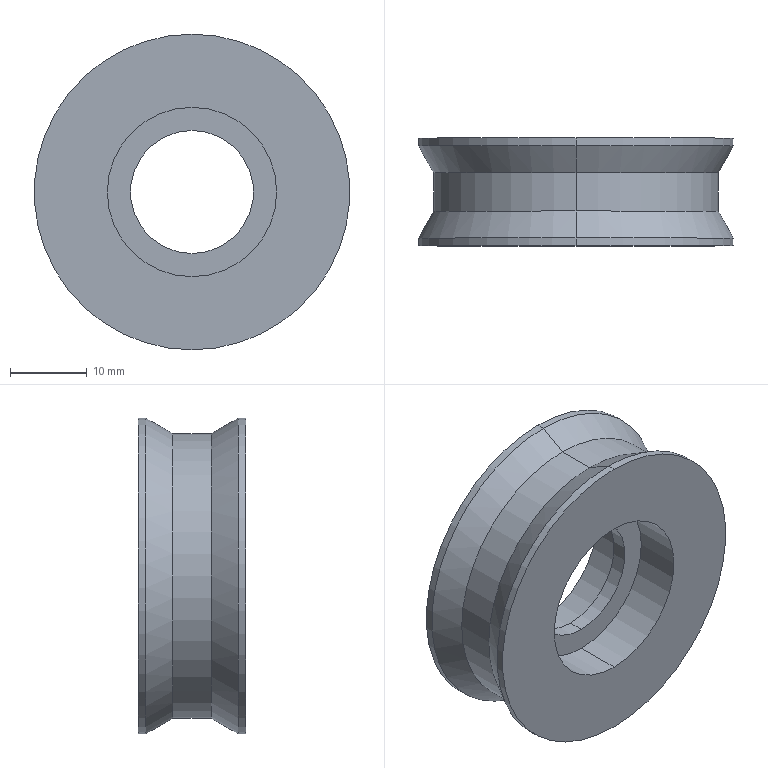Part | SolidWorks | features Revolution 1 | 1 solid | 20 faces | box 41 x 14 x 41 mm | volume 11422 mm3 | cylinder 12 | cone 4 | plane 4 | commonest cylinder face diameters 22 x4 41 x4 16 x2 37 x2
STEP:
#1=CARTESIAN_POINT('',(0.,1.,-11.));
#2=VERTEX_POINT('',#1);
#3=CARTESIAN_POINT('',(0.,1.,11.));
#4=VERTEX_POINT('',#3);
#5=CARTESIAN_POINT('',(0.,1.,0.));
#6=DIRECTION('',(0.,1.,0.));
#7=DIRECTION('',(0.,0.,1.));
#8=AXIS2_PLACEMENT_3D('',#5,#6,#7);
#9=CIRCLE('',#8,11.);
#10=EDGE_CURVE('',#2,#4,#9,.T.);
#11=ORIENTED_EDGE('',*,*,#10,.F.);
#12=CARTESIAN_POINT('',(0.,7.,-11.));
#13=VERTEX_POINT('',#12);
#14=CARTESIAN_POINT('',(0.,20.639,-11.));
#15=DIRECTION('',(0.,1.,0.));
#16=VECTOR('',#15,1000.);
#17=LINE('',#14,#16);
#18=EDGE_CURVE('',#2,#13,#17,.T.);
#19=ORIENTED_EDGE('',*,*,#18,.T.);
#20=CARTESIAN_POINT('',(0.,7.,11.));
#21=VERTEX_POINT('',#20);
#22=CARTESIAN_POINT('',(0.,7.,0.));
#23=DIRECTION('',(0.,1.,0.));
#24=DIRECTION('',(0.,0.,1.));
#25=AXIS2_PLACEMENT_3D('',#22,#23,#24);
#26=CIRCLE('',#25,11.);
#27=EDGE_CURVE('',#13,#21,#26,.T.);
#28=ORIENTED_EDGE('',*,*,#27,.T.);
#29=CARTESIAN_POINT('',(0.,20.639,11.));
#30=DIRECTION('',(0.,1.,0.));
#31=VECTOR('',#30,1000.);
#32=LINE('',#29,#31);
#33=EDGE_CURVE('',#4,#21,#32,.T.);
#34=ORIENTED_EDGE('',*,*,#33,.F.);
#35=EDGE_LOOP('',(#11,#19,#28,#34));
#36=FACE_OUTER_BOUND('',#35,.T.);
#37=CARTESIAN_POINT('',(0.,20.639,0.));
#38=DIRECTION('',(0.,1.,0.));
#39=DIRECTION('',(0.,0.,1.));
#40=AXIS2_PLACEMENT_3D('',#37,#38,#39);
#41=CYLINDRICAL_SURFACE('',#40,11.);
#42=ADVANCED_FACE('',(#36),#41,.F.);
#43=CARTESIAN_POINT('',(0.,-1.,-8.));
#44=VERTEX_POINT('',#43);
#45=CARTESIAN_POINT('',(0.,-1.,8.));
#46=VERTEX_POINT('',#45);
#47=CARTESIAN_POINT('',(0.,-1.,0.));
#48=DIRECTION('',(0.,1.,0.));
#49=DIRECTION('',(0.,0.,1.));
#50=AXIS2_PLACEMENT_3D('',#47,#48,#49);
#51=CIRCLE('',#50,8.);
#52=EDGE_CURVE('',#44,#46,#51,.T.);
#53=ORIENTED_EDGE('',*,*,#52,.F.);
#54=CARTESIAN_POINT('',(0.,1.,-8.));
#55=VERTEX_POINT('',#54);
#56=CARTESIAN_POINT('',(0.,20.639,-8.));
#57=DIRECTION('',(0.,1.,0.));
#58=VECTOR('',#57,1000.);
#59=LINE('',#56,#58);
#60=EDGE_CURVE('',#44,#55,#59,.T.);
#61=ORIENTED_EDGE('',*,*,#60,.T.);
#62=CARTESIAN_POINT('',(0.,1.,8.));
#63=VERTEX_POINT('',#62);
#64=CARTESIAN_POINT('',(0.,1.,0.));
#65=DIRECTION('',(0.,1.,0.));
#66=DIRECTION('',(0.,0.,1.));
#67=AXIS2_PLACEMENT_3D('',#64,#65,#66);
#68=CIRCLE('',#67,8.);
#69=EDGE_CURVE('',#55,#63,#68,.T.);
#70=ORIENTED_EDGE('',*,*,#69,.T.);
#71=CARTESIAN_POINT('',(0.,20.639,8.));
#72=DIRECTION('',(0.,1.,0.));
#73=VECTOR('',#72,1000.);
#74=LINE('',#71,#73);
#75=EDGE_CURVE('',#46,#63,#74,.T.);
#76=ORIENTED_EDGE('',*,*,#75,.F.);
#77=EDGE_LOOP('',(#53,#61,#70,#76));
#78=FACE_OUTER_BOUND('',#77,.T.);
#79=CARTESIAN_POINT('',(0.,20.639,0.));
#80=DIRECTION('',(0.,1.,0.));
#81=DIRECTION('',(0.,0.,1.));
#82=AXIS2_PLACEMENT_3D('',#79,#80,#81);
#83=CYLINDRICAL_SURFACE('',#82,8.);
#84=ADVANCED_FACE('',(#78),#83,.F.);
#85=CARTESIAN_POINT('',(0.,-7.,-11.));
#86=VERTEX_POINT('',#85);
#87=CARTESIAN_POINT('',(0.,-7.,11.));
#88=VERTEX_POINT('',#87);
#89=CARTESIAN_POINT('',(0.,-7.,0.));
#90=DIRECTION('',(0.,1.,0.));
#91=DIRECTION('',(0.,0.,1.));
#92=AXIS2_PLACEMENT_3D('',#89,#90,#91);
#93=CIRCLE('',#92,11.);
#94=EDGE_CURVE('',#86,#88,#93,.T.);
#95=ORIENTED_EDGE('',*,*,#94,.F.);
#96=CARTESIAN_POINT('',(0.,-1.,-11.));
#97=VERTEX_POINT('',#96);
#98=CARTESIAN_POINT('',(0.,20.639,-11.));
#99=DIRECTION('',(0.,1.,0.));
#100=VECTOR('',#99,1000.);
#101=LINE('',#98,#100);
#102=EDGE_CURVE('',#86,#97,#101,.T.);
#103=ORIENTED_EDGE('',*,*,#102,.T.);
#104=CARTESIAN_POINT('',(0.,-1.,11.));
#105=VERTEX_POINT('',#104);
#106=CARTESIAN_POINT('',(0.,-1.,0.));
#107=DIRECTION('',(0.,1.,0.));
#108=DIRECTION('',(0.,0.,1.));
#109=AXIS2_PLACEMENT_3D('',#106,#107,#108);
#110=CIRCLE('',#109,11.);
#111=EDGE_CURVE('',#97,#105,#110,.T.);
#112=ORIENTED_EDGE('',*,*,#111,.T.);
#113=CARTESIAN_POINT('',(0.,20.639,11.));
#114=DIRECTION('',(0.,1.,0.));
#115=VECTOR('',#114,1000.);
#116=LINE('',#113,#115);
#117=EDGE_CURVE('',#88,#105,#116,.T.);
#118=ORIENTED_EDGE('',*,*,#117,.F.);
#119=EDGE_LOOP('',(#95,#103,#112,#118));
#120=FACE_OUTER_BOUND('',#119,.T.);
#121=CARTESIAN_POINT('',(0.,20.639,0.));
#122=DIRECTION('',(0.,1.,0.));
#123=DIRECTION('',(0.,0.,1.));
#124=AXIS2_PLACEMENT_3D('',#121,#122,#123);
#125=CYLINDRICAL_SURFACE('',#124,11.);
#126=ADVANCED_FACE('',(#120),#125,.F.);
#127=CARTESIAN_POINT('',(0.,-7.,20.5));
#128=VERTEX_POINT('',#127);
#129=CARTESIAN_POINT('',(0.,-7.,-20.5));
#130=VERTEX_POINT('',#129);
#131=CARTESIAN_POINT('',(0.,-7.,0.));
#132=DIRECTION('',(0.,1.,0.));
#133=DIRECTION('',(0.,0.,1.));
#134=AXIS2_PLACEMENT_3D('',#131,#132,#133);
#135=CIRCLE('',#134,20.5);
#136=EDGE_CURVE('',#128,#130,#135,.T.);
#137=ORIENTED_EDGE('',*,*,#136,.T.);
#138=CARTESIAN_POINT('',(0.,-6.,-20.5));
#139=VERTEX_POINT('',#138);
#140=CARTESIAN_POINT('',(0.,20.639,-20.5));
#141=DIRECTION('',(0.,1.,0.));
#142=VECTOR('',#141,1000.);
#143=LINE('',#140,#142);
#144=EDGE_CURVE('',#130,#139,#143,.T.);
#145=ORIENTED_EDGE('',*,*,#144,.T.);
#146=CARTESIAN_POINT('',(0.,-6.,20.5));
#147=VERTEX_POINT('',#146);
#148=CARTESIAN_POINT('',(0.,-6.,0.));
#149=DIRECTION('',(0.,1.,0.));
#150=DIRECTION('',(0.,0.,1.));
#151=AXIS2_PLACEMENT_3D('',#148,#149,#150);
#152=CIRCLE('',#151,20.5);
#153=EDGE_CURVE('',#147,#139,#152,.T.);
#154=ORIENTED_EDGE('',*,*,#153,.F.);
#155=CARTESIAN_POINT('',(0.,20.639,20.5));
#156=DIRECTION('',(0.,1.,0.));
#157=VECTOR('',#156,1000.);
#158=LINE('',#155,#157);
#159=EDGE_CURVE('',#128,#147,#158,.T.);
#160=ORIENTED_EDGE('',*,*,#159,.F.);
#161=EDGE_LOOP('',(#137,#145,#154,#160));
#162=FACE_OUTER_BOUND('',#161,.T.);
#163=CARTESIAN_POINT('',(0.,20.639,0.));
#164=DIRECTION('',(0.,1.,0.));
#165=DIRECTION('',(0.,0.,1.));
#166=AXIS2_PLACEMENT_3D('',#163,#164,#165);
#167=CYLINDRICAL_SURFACE('',#166,20.5);
#168=ADVANCED_FACE('',(#162),#167,.T.);
#169=CARTESIAN_POINT('',(0.,-2.5,18.5));
#170=VERTEX_POINT('',#169);
#171=CARTESIAN_POINT('',(0.,-2.5,-18.5));
#172=VERTEX_POINT('',#171);
#173=CARTESIAN_POINT('',(0.,-2.5,0.));
#174=DIRECTION('',(0.,1.,0.));
#175=DIRECTION('',(0.,0.,1.));
#176=AXIS2_PLACEMENT_3D('',#173,#174,#175);
#177=CIRCLE('',#176,18.5);
#178=EDGE_CURVE('',#170,#172,#177,.T.);
#179=ORIENTED_EDGE('',*,*,#178,.F.);
#180=CARTESIAN_POINT('',(0.,-6.,20.5));
#181=DIRECTION('',(0.,-0.8682,0.4961));
#182=VECTOR('',#181,1000.);
#183=LINE('',#180,#182);
#184=EDGE_CURVE('',#170,#147,#183,.T.);
#185=ORIENTED_EDGE('',*,*,#184,.T.);
#186=ORIENTED_EDGE('',*,*,#153,.T.);
#187=CARTESIAN_POINT('',(0.,-6.,-20.5));
#188=DIRECTION('',(0.,-0.8682,-0.4961));
#189=VECTOR('',#188,1000.);
#190=LINE('',#187,#189);
#191=EDGE_CURVE('',#172,#139,#190,.T.);
#192=ORIENTED_EDGE('',*,*,#191,.F.);
#193=EDGE_LOOP('',(#179,#185,#186,#192));
#194=FACE_OUTER_BOUND('',#193,.T.);
#195=CARTESIAN_POINT('',(0.,-6.,0.));
#196=DIRECTION('',(0.,-1.,0.));
#197=DIRECTION('',(0.,0.,-1.));
#198=AXIS2_PLACEMENT_3D('',#195,#196,#197);
#199=CONICAL_SURFACE('',#198,20.5,0.5191);
#200=ADVANCED_FACE('',(#194),#199,.T.);
#201=ORIENTED_EDGE('',*,*,#178,.T.);
#202=CARTESIAN_POINT('',(0.,2.5,-18.5));
#203=VERTEX_POINT('',#202);
#204=CARTESIAN_POINT('',(0.,20.639,-18.5));
#205=DIRECTION('',(0.,1.,0.));
#206=VECTOR('',#205,1000.);
#207=LINE('',#204,#206);
#208=EDGE_CURVE('',#172,#203,#207,.T.);
#209=ORIENTED_EDGE('',*,*,#208,.T.);
#210=CARTESIAN_POINT('',(0.,2.5,18.5));
#211=VERTEX_POINT('',#210);
#212=CARTESIAN_POINT('',(0.,2.5,0.));
#213=DIRECTION('',(0.,1.,0.));
#214=DIRECTION('',(0.,0.,1.));
#215=AXIS2_PLACEMENT_3D('',#212,#213,#214);
#216=CIRCLE('',#215,18.5);
#217=EDGE_CURVE('',#211,#203,#216,.T.);
#218=ORIENTED_EDGE('',*,*,#217,.F.);
#219=CARTESIAN_POINT('',(0.,20.639,18.5));
#220=DIRECTION('',(0.,1.,0.));
#221=VECTOR('',#220,1000.);
#222=LINE('',#219,#221);
#223=EDGE_CURVE('',#170,#211,#222,.T.);
#224=ORIENTED_EDGE('',*,*,#223,.F.);
#225=EDGE_LOOP('',(#201,#209,#218,#224));
#226=FACE_OUTER_BOUND('',#225,.T.);
#227=CARTESIAN_POINT('',(0.,20.639,0.));
#228=DIRECTION('',(0.,1.,0.));
#229=DIRECTION('',(0.,0.,1.));
#230=AXIS2_PLACEMENT_3D('',#227,#228,#229);
#231=CYLINDRICAL_SURFACE('',#230,18.5);
#232=ADVANCED_FACE('',(#226),#231,.T.);
#233=ORIENTED_EDGE('',*,*,#217,.T.);
#234=CARTESIAN_POINT('',(0.,6.,-20.5));
#235=VERTEX_POINT('',#234);
#236=CARTESIAN_POINT('',(0.,2.5,-18.5));
#237=DIRECTION('',(0.,0.8682,-0.4961));
#238=VECTOR('',#237,1000.);
#239=LINE('',#236,#238);
#240=EDGE_CURVE('',#203,#235,#239,.T.);
#241=ORIENTED_EDGE('',*,*,#240,.T.);
#242=CARTESIAN_POINT('',(0.,6.,20.5));
#243=VERTEX_POINT('',#242);
#244=CARTESIAN_POINT('',(0.,6.,0.));
#245=DIRECTION('',(0.,1.,0.));
#246=DIRECTION('',(0.,0.,1.));
#247=AXIS2_PLACEMENT_3D('',#244,#245,#246);
#248=CIRCLE('',#247,20.5);
#249=EDGE_CURVE('',#243,#235,#248,.T.);
#250=ORIENTED_EDGE('',*,*,#249,.F.);
#251=CARTESIAN_POINT('',(0.,2.5,18.5));
#252=DIRECTION('',(0.,0.8682,0.4961));
#253=VECTOR('',#252,1000.);
#254=LINE('',#251,#253);
#255=EDGE_CURVE('',#211,#243,#254,.T.);
#256=ORIENTED_EDGE('',*,*,#255,.F.);
#257=EDGE_LOOP('',(#233,#241,#250,#256));
#258=FACE_OUTER_BOUND('',#257,.T.);
#259=CARTESIAN_POINT('',(0.,2.5,0.));
#260=DIRECTION('',(0.,1.,0.));
#261=DIRECTION('',(0.,0.,1.));
#262=AXIS2_PLACEMENT_3D('',#259,#260,#261);
#263=CONICAL_SURFACE('',#262,18.5,0.5191);
#264=ADVANCED_FACE('',(#258),#263,.T.);
#265=ORIENTED_EDGE('',*,*,#249,.T.);
#266=CARTESIAN_POINT('',(0.,7.,-20.5));
#267=VERTEX_POINT('',#266);
#268=CARTESIAN_POINT('',(0.,20.639,-20.5));
#269=DIRECTION('',(0.,1.,0.));
#270=VECTOR('',#269,1000.);
#271=LINE('',#268,#270);
#272=EDGE_CURVE('',#235,#267,#271,.T.);
#273=ORIENTED_EDGE('',*,*,#272,.T.);
#274=CARTESIAN_POINT('',(0.,7.,20.5));
#275=VERTEX_POINT('',#274);
#276=CARTESIAN_POINT('',(0.,7.,0.));
#277=DIRECTION('',(0.,1.,0.));
#278=DIRECTION('',(0.,0.,1.));
#279=AXIS2_PLACEMENT_3D('',#276,#277,#278);
#280=CIRCLE('',#279,20.5);
#281=EDGE_CURVE('',#275,#267,#280,.T.);
#282=ORIENTED_EDGE('',*,*,#281,.F.);
#283=CARTESIAN_POINT('',(0.,20.639,20.5));
#284=DIRECTION('',(0.,1.,0.));
#285=VECTOR('',#284,1000.);
#286=LINE('',#283,#285);
#287=EDGE_CURVE('',#243,#275,#286,.T.);
#288=ORIENTED_EDGE('',*,*,#287,.F.);
#289=EDGE_LOOP('',(#265,#273,#282,#288));
#290=FACE_OUTER_BOUND('',#289,.T.);
#291=CARTESIAN_POINT('',(0.,20.639,0.));
#292=DIRECTION('',(0.,1.,0.));
#293=DIRECTION('',(0.,0.,1.));
#294=AXIS2_PLACEMENT_3D('',#291,#292,#293);
#295=CYLINDRICAL_SURFACE('',#294,20.5);
#296=ADVANCED_FACE('',(#290),#295,.T.);
#297=ORIENTED_EDGE('',*,*,#272,.F.);
#298=CARTESIAN_POINT('',(0.,6.,0.));
#299=DIRECTION('',(0.,1.,0.));
#300=DIRECTION('',(0.,0.,1.));
#301=AXIS2_PLACEMENT_3D('',#298,#299,#300);
#302=CIRCLE('',#301,20.5);
#303=EDGE_CURVE('',#235,#243,#302,.T.);
#304=ORIENTED_EDGE('',*,*,#303,.T.);
#305=ORIENTED_EDGE('',*,*,#287,.T.);
#306=CARTESIAN_POINT('',(0.,7.,0.));
#307=DIRECTION('',(0.,1.,0.));
#308=DIRECTION('',(0.,0.,1.));
#309=AXIS2_PLACEMENT_3D('',#306,#307,#308);
#310=CIRCLE('',#309,20.5);
#311=EDGE_CURVE('',#267,#275,#310,.T.);
#312=ORIENTED_EDGE('',*,*,#311,.F.);
#313=EDGE_LOOP('',(#297,#304,#305,#312));
#314=FACE_OUTER_BOUND('',#313,.T.);
#315=CARTESIAN_POINT('',(0.,20.639,0.));
#316=DIRECTION('',(0.,1.,0.));
#317=DIRECTION('',(0.,0.,1.));
#318=AXIS2_PLACEMENT_3D('',#315,#316,#317);
#319=CYLINDRICAL_SURFACE('',#318,20.5);
#320=ADVANCED_FACE('',(#314),#319,.T.);
#321=ORIENTED_EDGE('',*,*,#240,.F.);
#322=CARTESIAN_POINT('',(0.,2.5,0.));
#323=DIRECTION('',(0.,1.,0.));
#324=DIRECTION('',(0.,0.,1.));
#325=AXIS2_PLACEMENT_3D('',#322,#323,#324);
#326=CIRCLE('',#325,18.5);
#327=EDGE_CURVE('',#203,#211,#326,.T.);
#328=ORIENTED_EDGE('',*,*,#327,.T.);
#329=ORIENTED_EDGE('',*,*,#255,.T.);
#330=ORIENTED_EDGE('',*,*,#303,.F.);
#331=EDGE_LOOP('',(#321,#328,#329,#330));
#332=FACE_OUTER_BOUND('',#331,.T.);
#333=CARTESIAN_POINT('',(0.,2.5,0.));
#334=DIRECTION('',(0.,1.,0.));
#335=DIRECTION('',(0.,0.,1.));
#336=AXIS2_PLACEMENT_3D('',#333,#334,#335);
#337=CONICAL_SURFACE('',#336,18.5,0.5191);
#338=ADVANCED_FACE('',(#332),#337,.T.);
#339=ORIENTED_EDGE('',*,*,#208,.F.);
#340=CARTESIAN_POINT('',(0.,-2.5,0.));
#341=DIRECTION('',(0.,1.,0.));
#342=DIRECTION('',(0.,0.,1.));
#343=AXIS2_PLACEMENT_3D('',#340,#341,#342);
#344=CIRCLE('',#343,18.5);
#345=EDGE_CURVE('',#172,#170,#344,.T.);
#346=ORIENTED_EDGE('',*,*,#345,.T.);
#347=ORIENTED_EDGE('',*,*,#223,.T.);
#348=ORIENTED_EDGE('',*,*,#327,.F.);
#349=EDGE_LOOP('',(#339,#346,#347,#348));
#350=FACE_OUTER_BOUND('',#349,.T.);
#351=CARTESIAN_POINT('',(0.,20.639,0.));
#352=DIRECTION('',(0.,1.,0.));
#353=DIRECTION('',(0.,0.,1.));
#354=AXIS2_PLACEMENT_3D('',#351,#352,#353);
#355=CYLINDRICAL_SURFACE('',#354,18.5);
#356=ADVANCED_FACE('',(#350),#355,.T.);
#357=ORIENTED_EDGE('',*,*,#184,.F.);
#358=ORIENTED_EDGE('',*,*,#345,.F.);
#359=ORIENTED_EDGE('',*,*,#191,.T.);
#360=CARTESIAN_POINT('',(0.,-6.,0.));
#361=DIRECTION('',(0.,1.,0.));
#362=DIRECTION('',(0.,0.,1.));
#363=AXIS2_PLACEMENT_3D('',#360,#361,#362);
#364=CIRCLE('',#363,20.5);
#365=EDGE_CURVE('',#139,#147,#364,.T.);
#366=ORIENTED_EDGE('',*,*,#365,.T.);
#367=EDGE_LOOP('',(#357,#358,#359,#366));
#368=FACE_OUTER_BOUND('',#367,.T.);
#369=CARTESIAN_POINT('',(0.,-6.,0.));
#370=DIRECTION('',(0.,-1.,0.));
#371=DIRECTION('',(0.,0.,-1.));
#372=AXIS2_PLACEMENT_3D('',#369,#370,#371);
#373=CONICAL_SURFACE('',#372,20.5,0.5191);
#374=ADVANCED_FACE('',(#368),#373,.T.);
#375=ORIENTED_EDGE('',*,*,#144,.F.);
#376=CARTESIAN_POINT('',(0.,-7.,0.));
#377=DIRECTION('',(0.,1.,0.));
#378=DIRECTION('',(0.,0.,1.));
#379=AXIS2_PLACEMENT_3D('',#376,#377,#378);
#380=CIRCLE('',#379,20.5);
#381=EDGE_CURVE('',#130,#128,#380,.T.);
#382=ORIENTED_EDGE('',*,*,#381,.T.);
#383=ORIENTED_EDGE('',*,*,#159,.T.);
#384=ORIENTED_EDGE('',*,*,#365,.F.);
#385=EDGE_LOOP('',(#375,#382,#383,#384));
#386=FACE_OUTER_BOUND('',#385,.T.);
#387=CARTESIAN_POINT('',(0.,20.639,0.));
#388=DIRECTION('',(0.,1.,0.));
#389=DIRECTION('',(0.,0.,1.));
#390=AXIS2_PLACEMENT_3D('',#387,#388,#389);
#391=CYLINDRICAL_SURFACE('',#390,20.5);
#392=ADVANCED_FACE('',(#386),#391,.T.);
#393=ORIENTED_EDGE('',*,*,#136,.F.);
#394=ORIENTED_EDGE('',*,*,#381,.F.);
#395=EDGE_LOOP('',(#393,#394));
#396=FACE_OUTER_BOUND('',#395,.T.);
#397=CARTESIAN_POINT('',(0.,-7.,0.));
#398=DIRECTION('',(0.,1.,0.));
#399=DIRECTION('',(0.,0.,1.));
#400=AXIS2_PLACEMENT_3D('',#397,#398,#399);
#401=CIRCLE('',#400,11.);
#402=EDGE_CURVE('',#88,#86,#401,.T.);
#403=ORIENTED_EDGE('',*,*,#402,.T.);
#404=ORIENTED_EDGE('',*,*,#94,.T.);
#405=EDGE_LOOP('',(#403,#404));
#406=FACE_BOUND('',#405,.T.);
#407=CARTESIAN_POINT('',(11.,-7.,0.));
#408=DIRECTION('',(0.,1.,0.));
#409=DIRECTION('',(0.,0.,1.));
#410=AXIS2_PLACEMENT_3D('',#407,#408,#409);
#411=PLANE('',#410);
#412=ADVANCED_FACE('',(#396,#406),#411,.F.);
#413=ORIENTED_EDGE('',*,*,#102,.F.);
#414=ORIENTED_EDGE('',*,*,#402,.F.);
#415=ORIENTED_EDGE('',*,*,#117,.T.);
#416=CARTESIAN_POINT('',(0.,-1.,0.));
#417=DIRECTION('',(0.,1.,0.));
#418=DIRECTION('',(0.,0.,1.));
#419=AXIS2_PLACEMENT_3D('',#416,#417,#418);
#420=CIRCLE('',#419,11.);
#421=EDGE_CURVE('',#105,#97,#420,.T.);
#422=ORIENTED_EDGE('',*,*,#421,.T.);
#423=EDGE_LOOP('',(#413,#414,#415,#422));
#424=FACE_OUTER_BOUND('',#423,.T.);
#425=CARTESIAN_POINT('',(0.,20.639,0.));
#426=DIRECTION('',(0.,1.,0.));
#427=DIRECTION('',(0.,0.,1.));
#428=AXIS2_PLACEMENT_3D('',#425,#426,#427);
#429=CYLINDRICAL_SURFACE('',#428,11.);
#430=ADVANCED_FACE('',(#424),#429,.F.);
#431=ORIENTED_EDGE('',*,*,#421,.F.);
#432=ORIENTED_EDGE('',*,*,#111,.F.);
#433=EDGE_LOOP('',(#431,#432));
#434=FACE_OUTER_BOUND('',#433,.T.);
#435=CARTESIAN_POINT('',(0.,-1.,0.));
#436=DIRECTION('',(0.,1.,0.));
#437=DIRECTION('',(0.,0.,1.));
#438=AXIS2_PLACEMENT_3D('',#435,#436,#437);
#439=CIRCLE('',#438,8.);
#440=EDGE_CURVE('',#46,#44,#439,.T.);
#441=ORIENTED_EDGE('',*,*,#440,.T.);
#442=ORIENTED_EDGE('',*,*,#52,.T.);
#443=EDGE_LOOP('',(#441,#442));
#444=FACE_BOUND('',#443,.T.);
#445=CARTESIAN_POINT('',(11.,-1.,0.));
#446=DIRECTION('',(0.,1.,0.));
#447=DIRECTION('',(0.,0.,1.));
#448=AXIS2_PLACEMENT_3D('',#445,#446,#447);
#449=PLANE('',#448);
#450=ADVANCED_FACE('',(#434,#444),#449,.F.);
#451=ORIENTED_EDGE('',*,*,#60,.F.);
#452=ORIENTED_EDGE('',*,*,#440,.F.);
#453=ORIENTED_EDGE('',*,*,#75,.T.);
#454=CARTESIAN_POINT('',(0.,1.,0.));
#455=DIRECTION('',(0.,1.,0.));
#456=DIRECTION('',(0.,0.,1.));
#457=AXIS2_PLACEMENT_3D('',#454,#455,#456);
#458=CIRCLE('',#457,8.);
#459=EDGE_CURVE('',#63,#55,#458,.T.);
#460=ORIENTED_EDGE('',*,*,#459,.T.);
#461=EDGE_LOOP('',(#451,#452,#453,#460));
#462=FACE_OUTER_BOUND('',#461,.T.);
#463=CARTESIAN_POINT('',(0.,20.639,0.));
#464=DIRECTION('',(0.,1.,0.));
#465=DIRECTION('',(0.,0.,1.));
#466=AXIS2_PLACEMENT_3D('',#463,#464,#465);
#467=CYLINDRICAL_SURFACE('',#466,8.);
#468=ADVANCED_FACE('',(#462),#467,.F.);
#469=ORIENTED_EDGE('',*,*,#459,.F.);
#470=ORIENTED_EDGE('',*,*,#69,.F.);
#471=EDGE_LOOP('',(#469,#470));
#472=FACE_BOUND('',#471,.T.);
#473=CARTESIAN_POINT('',(0.,1.,0.));
#474=DIRECTION('',(0.,1.,0.));
#475=DIRECTION('',(0.,0.,1.));
#476=AXIS2_PLACEMENT_3D('',#473,#474,#475);
#477=CIRCLE('',#476,11.);
#478=EDGE_CURVE('',#4,#2,#477,.T.);
#479=ORIENTED_EDGE('',*,*,#478,.T.);
#480=ORIENTED_EDGE('',*,*,#10,.T.);
#481=EDGE_LOOP('',(#479,#480));
#482=FACE_OUTER_BOUND('',#481,.T.);
#483=CARTESIAN_POINT('',(8.,1.,0.));
#484=DIRECTION('',(0.,-1.,0.));
#485=DIRECTION('',(0.,0.,-1.));
#486=AXIS2_PLACEMENT_3D('',#483,#484,#485);
#487=PLANE('',#486);
#488=ADVANCED_FACE('',(#472,#482),#487,.F.);
#489=ORIENTED_EDGE('',*,*,#18,.F.);
#490=ORIENTED_EDGE('',*,*,#478,.F.);
#491=ORIENTED_EDGE('',*,*,#33,.T.);
#492=CARTESIAN_POINT('',(0.,7.,0.));
#493=DIRECTION('',(0.,1.,0.));
#494=DIRECTION('',(0.,0.,1.));
#495=AXIS2_PLACEMENT_3D('',#492,#493,#494);
#496=CIRCLE('',#495,11.);
#497=EDGE_CURVE('',#21,#13,#496,.T.);
#498=ORIENTED_EDGE('',*,*,#497,.T.);
#499=EDGE_LOOP('',(#489,#490,#491,#498));
#500=FACE_OUTER_BOUND('',#499,.T.);
#501=CARTESIAN_POINT('',(0.,20.639,0.));
#502=DIRECTION('',(0.,1.,0.));
#503=DIRECTION('',(0.,0.,1.));
#504=AXIS2_PLACEMENT_3D('',#501,#502,#503);
#505=CYLINDRICAL_SURFACE('',#504,11.);
#506=ADVANCED_FACE('',(#500),#505,.F.);
#507=ORIENTED_EDGE('',*,*,#497,.F.);
#508=ORIENTED_EDGE('',*,*,#27,.F.);
#509=EDGE_LOOP('',(#507,#508));
#510=FACE_BOUND('',#509,.T.);
#511=ORIENTED_EDGE('',*,*,#281,.T.);
#512=ORIENTED_EDGE('',*,*,#311,.T.);
#513=EDGE_LOOP('',(#511,#512));
#514=FACE_OUTER_BOUND('',#513,.T.);
#515=CARTESIAN_POINT('',(11.,7.,0.));
#516=DIRECTION('',(0.,-1.,0.));
#517=DIRECTION('',(0.,0.,-1.));
#518=AXIS2_PLACEMENT_3D('',#515,#516,#517);
#519=PLANE('',#518);
#520=ADVANCED_FACE('',(#510,#514),#519,.F.);
#521=CLOSED_SHELL('',(#42,#84,#126,#168,#200,#232,#264,#296,#320,#338,#356,#374,#392,#412,#430,#450,#468,#488,#506,#520));
#522=MANIFOLD_SOLID_BREP('',#521);
#523=CARTESIAN_POINT('',(0.,0.,0.));
#524=DIRECTION('',(0.,0.,1.));
#525=DIRECTION('',(1.,0.,0.));
#526=AXIS2_PLACEMENT_3D('',#523,#524,#525);
#527=(LENGTH_UNIT()NAMED_UNIT(*)SI_UNIT(.MILLI.,.METRE.));
#528=UNCERTAINTY_MEASURE_WITH_UNIT(LENGTH_MEASURE(0.00001),#527,'','');
#529=(NAMED_UNIT(*)PLANE_ANGLE_UNIT()SI_UNIT($,.RADIAN.));
#530=(NAMED_UNIT(*)SI_UNIT($,.STERADIAN.)SOLID_ANGLE_UNIT());
#531=(GEOMETRIC_REPRESENTATION_CONTEXT(3)GLOBAL_UNCERTAINTY_ASSIGNED_CONTEXT((#528))GLOBAL_UNIT_ASSIGNED_CONTEXT((#527,#529,#530))REPRESENTATION_CONTEXT('',''));
#532=ADVANCED_BREP_SHAPE_REPRESENTATION('',(#522,#526),#531);